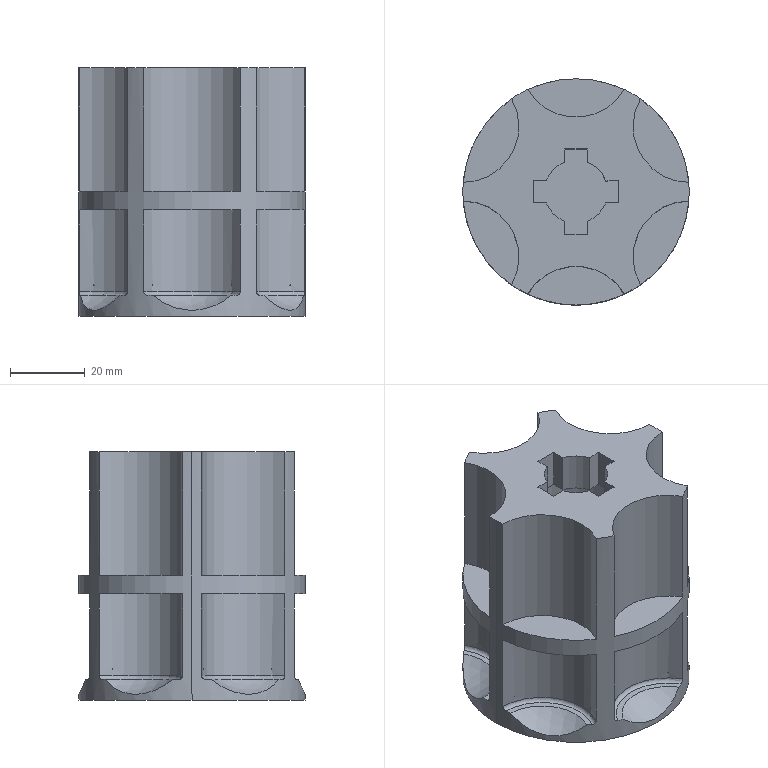Part | NX | features BREP 1 | 1 solid | 120 faces | box 60.7 x 60.7 x 66.6 mm | volume 88337 mm3 | plane 60 | cylinder 24 | sphere 18 | cone 12 | torus 6 | commonest cylinder face diameters 30 x12 17 x6 31 x4 60.7 x2